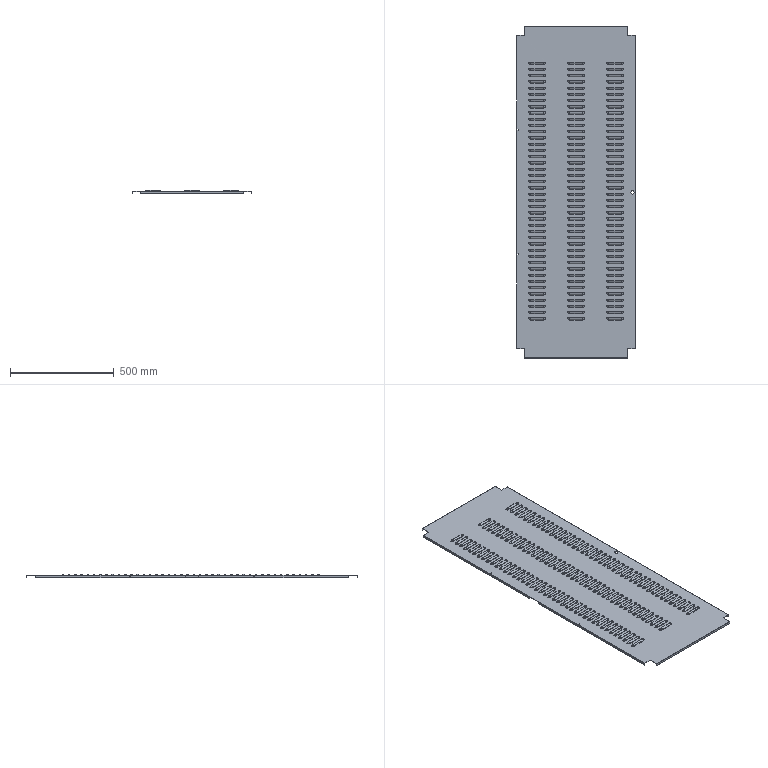Part | STEP file | 1 solid | 1842 faces | box 572.5 x 1598 x 16 mm | volume 960867 mm3 | cylinder 519 | torus 504 | sphere 504 | plane 315 | commonest cylinder face diameters 4 x126 6 x126 23 x126 25 x126 0.4 x7 2.4 x6